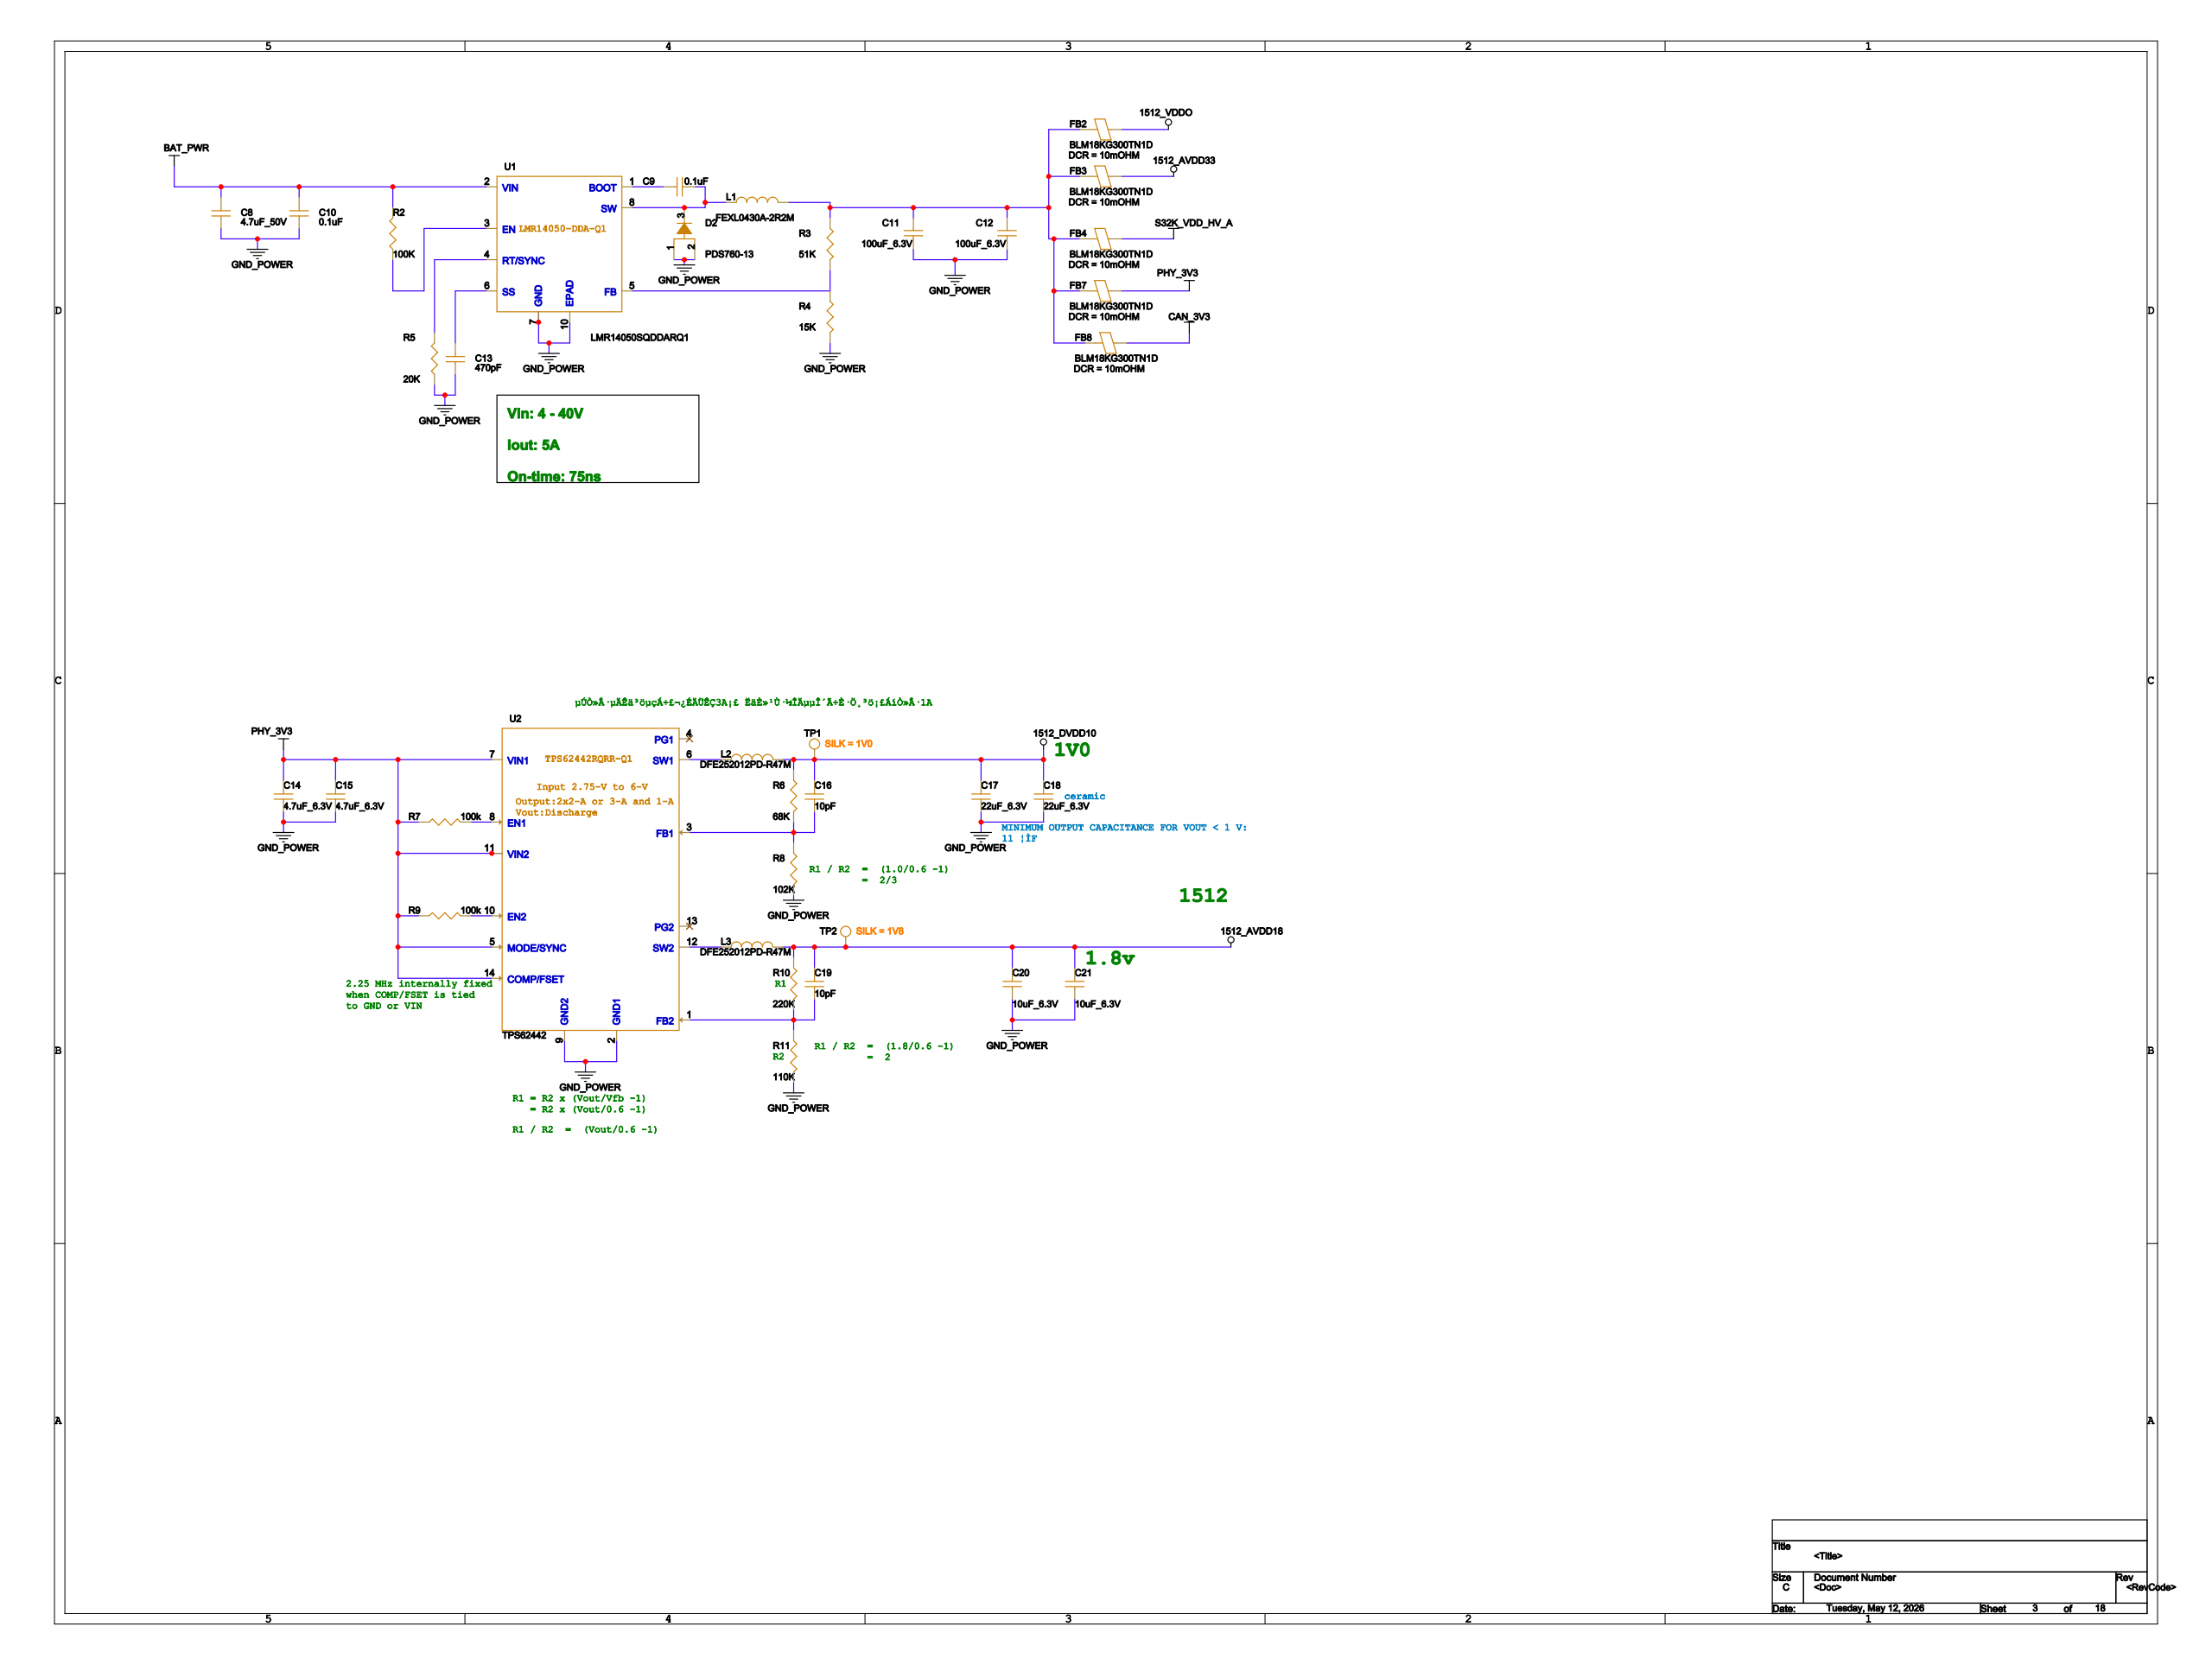Circuit board | Cadence Allegro | 330 parts | 215 nets | one sheet of the schematic
Parts on this sheet (reference | value | footprint):
C8 | 4.7uF_50V | 1210
C9 | 0.1uF | 0402
C10 | 0.1uF | 0402
C11 | 100uF_6.3V | 1206
C12 | 100uF_6.3V | 1206
C13 | 470pF | 0402
C14 | 4.7uF_6.3V | 0201
C15 | 4.7uF_6.3V | 0201
C16 | 10pF | 0201
C17 | 22uF_6.3V | 0402
C18 | 22uF_6.3V | 0402
C19 | 10pF | 0201
C20 | 10uF_6.3V | 0402
C21 | 10uF_6.3V | 0402
D2 | PDS760-13 | PDS760
FB2 | BLM18KG300TN1D | 0603
FB3 | BLM18KG300TN1D | 0603
FB4 | BLM18KG300TN1D | 0603
FB7 | BLM18KG300TN1D | 0603
FB8 | BLM18KG300TN1D | 0603
L1 | FEXL0430A-2R2M | L_41X41_H210_BOURNS
L2 | DFE252012PD-R47M | 1008
L3 | DFE252012PD-R47M | 1008
R2 | 100K | 0402
R3 | 51K | 0402
R4 | 15K | 0402
R5 | 20K | 0402
R6 | 68K | 0201
R7 | 100k | 0201
R8 | 102K | 0201
R9 | 100k | 0201
R10 | 220K | 0201
R11 | 110K | 0201
TP1 | TP | S0400CI
TP2 | TP | S0400CI
U1 | LMR14050SQDDARQ1 | SOP8P_60_PAD29X21_127_H170
U2 | TPS62442 | QFN14P_27X23_05_H100
Nets of these parts (net: part-pin ...):
CAN_3V3: FB8-1
BAT_GND: C8-1 C10-1 C11-2 C12-2 C13-1 C14-1 C15-1 C17-1 C18-1 C20-1 C21-1 D2-1 D2-2 R4-2 R5-1 R8-2 R11-2 U1-7 U1-10 U2-2 U2-9
PHY_3V3: C14-2 C15-2 FB7-1 R7-1 R9-1 U2-5 U2-7 U2-11 U2-14
N16918481: C16-1 R6-2 R8-1 U2-3
1512_DVDD10: C16-2 C17-2 C18-2 L2-2 R6-1 TP1-1
N16918668: C19-1 R10-2 R11-1 U2-1
1512_AVDD18: C19-2 C20-2 C21-2 L3-2 R10-1 TP2-1
S32K_VDD_HV_A: FB4-1
1512_AVDD33: FB3-1
1512_VDDO: FB2-1
BAT_PWR: C8-2 C10-2 R2-2 U1-2
N16918403: L2-1 U2-6
N16918608: L3-1 U2-12
N16918495: R7-2 U2-8
N16918566: R9-2 U2-10
N2240291: R2-1 U1-3
N2240371: R5-2 U1-4
N1797886: C11-1 C12-1 FB2-2 FB3-2 FB4-2 FB7-2 FB8-2 L1-2 R3-1
N2240407: R3-2 R4-1 U1-5
N2240129: C9-1 D2-3 L1-1 U1-8
N2240437: C13-2 U1-6
N2240125: C9-2 U1-1